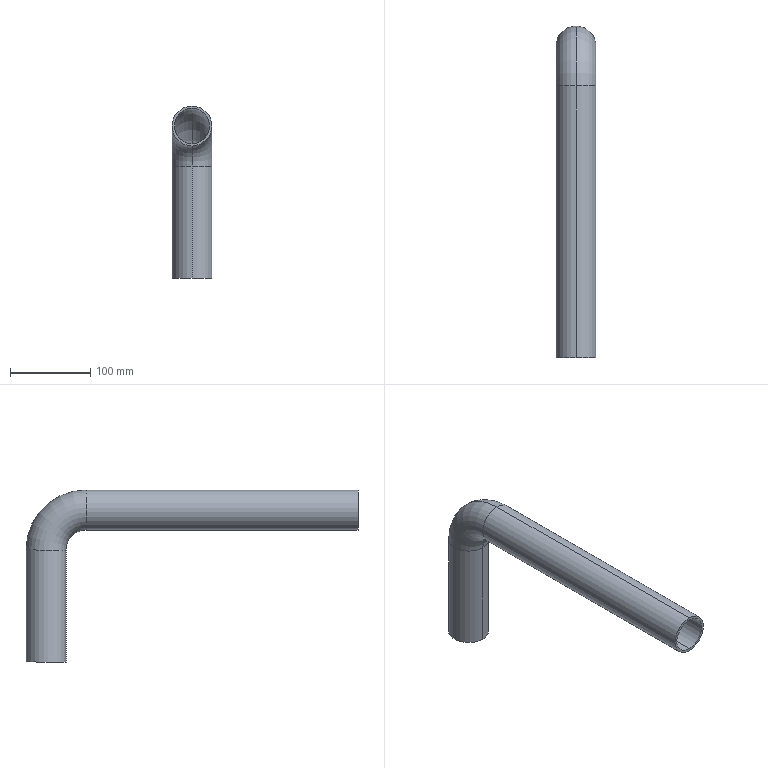Part | SolidWorks | features BaseBody 1 | 1 solid | 14 faces | box 50 x 415 x 215 mm | volume 247413 mm3 | cylinder 8 | torus 4 | plane 2 | commonest cylinder face diameters 44 x4 50 x4
STEP:
#1=CARTESIAN_POINT('',(0.,340.,-25.));
#2=VERTEX_POINT('',#1);
#3=CARTESIAN_POINT('',(0.,340.,25.));
#4=VERTEX_POINT('',#3);
#5=CARTESIAN_POINT('',(0.,340.,0.));
#6=DIRECTION('',(0.,1.,0.));
#7=DIRECTION('',(0.,0.,1.));
#8=AXIS2_PLACEMENT_3D('',#5,#6,#7);
#9=CIRCLE('',#8,25.);
#10=EDGE_CURVE('',#2,#4,#9,.T.);
#11=ORIENTED_EDGE('',*,*,#10,.T.);
#12=CARTESIAN_POINT('',(0.,415.,-50.));
#13=VERTEX_POINT('',#12);
#14=CARTESIAN_POINT('',(0.,340.,-50.));
#15=DIRECTION('',(-1.,0.,0.));
#16=DIRECTION('',(0.,0.,1.));
#17=AXIS2_PLACEMENT_3D('',#14,#15,#16);
#18=CIRCLE('',#17,75.);
#19=EDGE_CURVE('',#4,#13,#18,.T.);
#20=ORIENTED_EDGE('',*,*,#19,.T.);
#21=CARTESIAN_POINT('',(0.,365.,-50.));
#22=VERTEX_POINT('',#21);
#23=CARTESIAN_POINT('',(0.,390.,-50.));
#24=DIRECTION('',(0.,0.,-1.));
#25=DIRECTION('',(0.,1.,0.));
#26=AXIS2_PLACEMENT_3D('',#23,#24,#25);
#27=CIRCLE('',#26,25.);
#28=EDGE_CURVE('',#22,#13,#27,.T.);
#29=ORIENTED_EDGE('',*,*,#28,.F.);
#30=CARTESIAN_POINT('',(0.,340.,-50.));
#31=DIRECTION('',(-1.,0.,0.));
#32=DIRECTION('',(0.,0.,1.));
#33=AXIS2_PLACEMENT_3D('',#30,#31,#32);
#34=CIRCLE('',#33,25.);
#35=EDGE_CURVE('',#2,#22,#34,.T.);
#36=ORIENTED_EDGE('',*,*,#35,.F.);
#37=EDGE_LOOP('',(#11,#20,#29,#36));
#38=FACE_OUTER_BOUND('',#37,.T.);
#39=CARTESIAN_POINT('',(0.,340.,-50.));
#40=DIRECTION('',(-1.,0.,0.));
#41=DIRECTION('',(0.,0.,-1.));
#42=AXIS2_PLACEMENT_3D('',#39,#40,#41);
#43=TOROIDAL_SURFACE('',#42,50.,25.);
#44=ADVANCED_FACE('',(#38),#43,.T.);
#45=CARTESIAN_POINT('',(0.,340.,22.));
#46=VERTEX_POINT('',#45);
#47=CARTESIAN_POINT('',(0.,340.,-22.));
#48=VERTEX_POINT('',#47);
#49=CARTESIAN_POINT('',(0.,340.,0.));
#50=DIRECTION('',(0.,1.,0.));
#51=DIRECTION('',(0.,0.,1.));
#52=AXIS2_PLACEMENT_3D('',#49,#50,#51);
#53=CIRCLE('',#52,22.);
#54=EDGE_CURVE('',#46,#48,#53,.T.);
#55=ORIENTED_EDGE('',*,*,#54,.F.);
#56=CARTESIAN_POINT('',(0.,412.,-50.));
#57=VERTEX_POINT('',#56);
#58=CARTESIAN_POINT('',(0.,340.,-50.));
#59=DIRECTION('',(-1.,0.,0.));
#60=DIRECTION('',(0.,0.,1.));
#61=AXIS2_PLACEMENT_3D('',#58,#59,#60);
#62=CIRCLE('',#61,72.);
#63=EDGE_CURVE('',#46,#57,#62,.T.);
#64=ORIENTED_EDGE('',*,*,#63,.T.);
#65=CARTESIAN_POINT('',(0.,368.,-50.));
#66=VERTEX_POINT('',#65);
#67=CARTESIAN_POINT('',(0.,390.,-50.));
#68=DIRECTION('',(0.,0.,-1.));
#69=DIRECTION('',(0.,1.,0.));
#70=AXIS2_PLACEMENT_3D('',#67,#68,#69);
#71=CIRCLE('',#70,22.);
#72=EDGE_CURVE('',#57,#66,#71,.T.);
#73=ORIENTED_EDGE('',*,*,#72,.T.);
#74=CARTESIAN_POINT('',(0.,340.,-50.));
#75=DIRECTION('',(-1.,0.,0.));
#76=DIRECTION('',(0.,0.,1.));
#77=AXIS2_PLACEMENT_3D('',#74,#75,#76);
#78=CIRCLE('',#77,28.);
#79=EDGE_CURVE('',#48,#66,#78,.T.);
#80=ORIENTED_EDGE('',*,*,#79,.F.);
#81=EDGE_LOOP('',(#55,#64,#73,#80));
#82=FACE_OUTER_BOUND('',#81,.T.);
#83=CARTESIAN_POINT('',(0.,340.,-50.));
#84=DIRECTION('',(-1.,0.,0.));
#85=DIRECTION('',(0.,0.,-1.));
#86=AXIS2_PLACEMENT_3D('',#83,#84,#85);
#87=TOROIDAL_SURFACE('',#86,50.,22.);
#88=ADVANCED_FACE('',(#82),#87,.F.);
#89=ORIENTED_EDGE('',*,*,#28,.T.);
#90=CARTESIAN_POINT('',(0.,415.,-190.));
#91=VERTEX_POINT('',#90);
#92=CARTESIAN_POINT('',(0.,415.,-50.));
#93=DIRECTION('',(0.,0.,-1.));
#94=VECTOR('',#93,1000.);
#95=LINE('',#92,#94);
#96=EDGE_CURVE('',#13,#91,#95,.T.);
#97=ORIENTED_EDGE('',*,*,#96,.T.);
#98=CARTESIAN_POINT('',(0.,365.,-190.));
#99=VERTEX_POINT('',#98);
#100=CARTESIAN_POINT('',(0.,390.,-190.));
#101=DIRECTION('',(0.,0.,-1.));
#102=DIRECTION('',(0.,1.,0.));
#103=AXIS2_PLACEMENT_3D('',#100,#101,#102);
#104=CIRCLE('',#103,25.);
#105=EDGE_CURVE('',#99,#91,#104,.T.);
#106=ORIENTED_EDGE('',*,*,#105,.F.);
#107=CARTESIAN_POINT('',(0.,365.,-50.));
#108=DIRECTION('',(0.,0.,-1.));
#109=VECTOR('',#108,1000.);
#110=LINE('',#107,#109);
#111=EDGE_CURVE('',#22,#99,#110,.T.);
#112=ORIENTED_EDGE('',*,*,#111,.F.);
#113=EDGE_LOOP('',(#89,#97,#106,#112));
#114=FACE_OUTER_BOUND('',#113,.T.);
#115=CARTESIAN_POINT('',(0.,390.,-50.));
#116=DIRECTION('',(0.,0.,-1.));
#117=DIRECTION('',(0.,-1.,0.));
#118=AXIS2_PLACEMENT_3D('',#115,#116,#117);
#119=CYLINDRICAL_SURFACE('',#118,25.);
#120=ADVANCED_FACE('',(#114),#119,.T.);
#121=ORIENTED_EDGE('',*,*,#72,.F.);
#122=CARTESIAN_POINT('',(0.,412.,-190.));
#123=VERTEX_POINT('',#122);
#124=CARTESIAN_POINT('',(0.,412.,-50.));
#125=DIRECTION('',(0.,0.,-1.));
#126=VECTOR('',#125,1000.);
#127=LINE('',#124,#126);
#128=EDGE_CURVE('',#57,#123,#127,.T.);
#129=ORIENTED_EDGE('',*,*,#128,.T.);
#130=CARTESIAN_POINT('',(0.,368.,-190.));
#131=VERTEX_POINT('',#130);
#132=CARTESIAN_POINT('',(0.,390.,-190.));
#133=DIRECTION('',(0.,0.,-1.));
#134=DIRECTION('',(0.,1.,0.));
#135=AXIS2_PLACEMENT_3D('',#132,#133,#134);
#136=CIRCLE('',#135,22.);
#137=EDGE_CURVE('',#123,#131,#136,.T.);
#138=ORIENTED_EDGE('',*,*,#137,.T.);
#139=CARTESIAN_POINT('',(0.,368.,-50.));
#140=DIRECTION('',(0.,0.,-1.));
#141=VECTOR('',#140,1000.);
#142=LINE('',#139,#141);
#143=EDGE_CURVE('',#66,#131,#142,.T.);
#144=ORIENTED_EDGE('',*,*,#143,.F.);
#145=EDGE_LOOP('',(#121,#129,#138,#144));
#146=FACE_OUTER_BOUND('',#145,.T.);
#147=CARTESIAN_POINT('',(0.,390.,-50.));
#148=DIRECTION('',(0.,0.,-1.));
#149=DIRECTION('',(0.,-1.,0.));
#150=AXIS2_PLACEMENT_3D('',#147,#148,#149);
#151=CYLINDRICAL_SURFACE('',#150,22.);
#152=ADVANCED_FACE('',(#146),#151,.F.);
#153=ORIENTED_EDGE('',*,*,#54,.T.);
#154=CARTESIAN_POINT('',(0.,0.,-22.));
#155=VERTEX_POINT('',#154);
#156=CARTESIAN_POINT('',(0.,340.,-22.));
#157=DIRECTION('',(0.,-1.,0.));
#158=VECTOR('',#157,1000.);
#159=LINE('',#156,#158);
#160=EDGE_CURVE('',#48,#155,#159,.T.);
#161=ORIENTED_EDGE('',*,*,#160,.T.);
#162=CARTESIAN_POINT('',(0.,0.,22.));
#163=VERTEX_POINT('',#162);
#164=CARTESIAN_POINT('',(0.,0.,0.));
#165=DIRECTION('',(0.,1.,0.));
#166=DIRECTION('',(0.,0.,1.));
#167=AXIS2_PLACEMENT_3D('',#164,#165,#166);
#168=CIRCLE('',#167,22.);
#169=EDGE_CURVE('',#163,#155,#168,.T.);
#170=ORIENTED_EDGE('',*,*,#169,.F.);
#171=CARTESIAN_POINT('',(0.,340.,22.));
#172=DIRECTION('',(0.,-1.,0.));
#173=VECTOR('',#172,1000.);
#174=LINE('',#171,#173);
#175=EDGE_CURVE('',#46,#163,#174,.T.);
#176=ORIENTED_EDGE('',*,*,#175,.F.);
#177=EDGE_LOOP('',(#153,#161,#170,#176));
#178=FACE_OUTER_BOUND('',#177,.T.);
#179=CARTESIAN_POINT('',(0.,340.,0.));
#180=DIRECTION('',(0.,-1.,0.));
#181=DIRECTION('',(0.,0.,1.));
#182=AXIS2_PLACEMENT_3D('',#179,#180,#181);
#183=CYLINDRICAL_SURFACE('',#182,22.);
#184=ADVANCED_FACE('',(#178),#183,.F.);
#185=ORIENTED_EDGE('',*,*,#10,.F.);
#186=CARTESIAN_POINT('',(0.,0.,-25.));
#187=VERTEX_POINT('',#186);
#188=CARTESIAN_POINT('',(0.,340.,-25.));
#189=DIRECTION('',(0.,-1.,0.));
#190=VECTOR('',#189,1000.);
#191=LINE('',#188,#190);
#192=EDGE_CURVE('',#2,#187,#191,.T.);
#193=ORIENTED_EDGE('',*,*,#192,.T.);
#194=CARTESIAN_POINT('',(0.,0.,25.));
#195=VERTEX_POINT('',#194);
#196=CARTESIAN_POINT('',(0.,0.,0.));
#197=DIRECTION('',(0.,1.,0.));
#198=DIRECTION('',(0.,0.,1.));
#199=AXIS2_PLACEMENT_3D('',#196,#197,#198);
#200=CIRCLE('',#199,25.);
#201=EDGE_CURVE('',#187,#195,#200,.T.);
#202=ORIENTED_EDGE('',*,*,#201,.T.);
#203=CARTESIAN_POINT('',(0.,340.,25.));
#204=DIRECTION('',(0.,-1.,0.));
#205=VECTOR('',#204,1000.);
#206=LINE('',#203,#205);
#207=EDGE_CURVE('',#4,#195,#206,.T.);
#208=ORIENTED_EDGE('',*,*,#207,.F.);
#209=EDGE_LOOP('',(#185,#193,#202,#208));
#210=FACE_OUTER_BOUND('',#209,.T.);
#211=CARTESIAN_POINT('',(0.,340.,0.));
#212=DIRECTION('',(0.,-1.,0.));
#213=DIRECTION('',(0.,0.,1.));
#214=AXIS2_PLACEMENT_3D('',#211,#212,#213);
#215=CYLINDRICAL_SURFACE('',#214,25.);
#216=ADVANCED_FACE('',(#210),#215,.T.);
#217=CARTESIAN_POINT('',(0.,0.,0.));
#218=DIRECTION('',(0.,1.,0.));
#219=DIRECTION('',(0.,0.,1.));
#220=AXIS2_PLACEMENT_3D('',#217,#218,#219);
#221=CIRCLE('',#220,25.);
#222=EDGE_CURVE('',#195,#187,#221,.T.);
#223=ORIENTED_EDGE('',*,*,#222,.F.);
#224=ORIENTED_EDGE('',*,*,#201,.F.);
#225=EDGE_LOOP('',(#223,#224));
#226=FACE_OUTER_BOUND('',#225,.T.);
#227=ORIENTED_EDGE('',*,*,#169,.T.);
#228=CARTESIAN_POINT('',(0.,0.,0.));
#229=DIRECTION('',(0.,1.,0.));
#230=DIRECTION('',(0.,0.,1.));
#231=AXIS2_PLACEMENT_3D('',#228,#229,#230);
#232=CIRCLE('',#231,22.);
#233=EDGE_CURVE('',#155,#163,#232,.T.);
#234=ORIENTED_EDGE('',*,*,#233,.T.);
#235=EDGE_LOOP('',(#227,#234));
#236=FACE_BOUND('',#235,.T.);
#237=CARTESIAN_POINT('',(0.,0.,0.));
#238=DIRECTION('',(0.,1.,0.));
#239=DIRECTION('',(1.,0.,0.));
#240=AXIS2_PLACEMENT_3D('',#237,#238,#239);
#241=PLANE('',#240);
#242=ADVANCED_FACE('',(#226,#236),#241,.F.);
#243=ORIENTED_EDGE('',*,*,#105,.T.);
#244=CARTESIAN_POINT('',(0.,390.,-190.));
#245=DIRECTION('',(0.,0.,-1.));
#246=DIRECTION('',(0.,1.,0.));
#247=AXIS2_PLACEMENT_3D('',#244,#245,#246);
#248=CIRCLE('',#247,25.);
#249=EDGE_CURVE('',#91,#99,#248,.T.);
#250=ORIENTED_EDGE('',*,*,#249,.T.);
#251=EDGE_LOOP('',(#243,#250));
#252=FACE_OUTER_BOUND('',#251,.T.);
#253=CARTESIAN_POINT('',(0.,390.,-190.));
#254=DIRECTION('',(0.,0.,-1.));
#255=DIRECTION('',(0.,1.,0.));
#256=AXIS2_PLACEMENT_3D('',#253,#254,#255);
#257=CIRCLE('',#256,22.);
#258=EDGE_CURVE('',#131,#123,#257,.T.);
#259=ORIENTED_EDGE('',*,*,#258,.F.);
#260=ORIENTED_EDGE('',*,*,#137,.F.);
#261=EDGE_LOOP('',(#259,#260));
#262=FACE_BOUND('',#261,.T.);
#263=CARTESIAN_POINT('',(0.,390.,-190.));
#264=DIRECTION('',(0.,0.,-1.));
#265=DIRECTION('',(-1.,0.,0.));
#266=AXIS2_PLACEMENT_3D('',#263,#264,#265);
#267=PLANE('',#266);
#268=ADVANCED_FACE('',(#252,#262),#267,.T.);
#269=ORIENTED_EDGE('',*,*,#192,.F.);
#270=CARTESIAN_POINT('',(0.,340.,0.));
#271=DIRECTION('',(0.,1.,0.));
#272=DIRECTION('',(0.,0.,1.));
#273=AXIS2_PLACEMENT_3D('',#270,#271,#272);
#274=CIRCLE('',#273,25.);
#275=EDGE_CURVE('',#4,#2,#274,.T.);
#276=ORIENTED_EDGE('',*,*,#275,.F.);
#277=ORIENTED_EDGE('',*,*,#207,.T.);
#278=ORIENTED_EDGE('',*,*,#222,.T.);
#279=EDGE_LOOP('',(#269,#276,#277,#278));
#280=FACE_OUTER_BOUND('',#279,.T.);
#281=CARTESIAN_POINT('',(0.,340.,0.));
#282=DIRECTION('',(0.,-1.,0.));
#283=DIRECTION('',(0.,0.,1.));
#284=AXIS2_PLACEMENT_3D('',#281,#282,#283);
#285=CYLINDRICAL_SURFACE('',#284,25.);
#286=ADVANCED_FACE('',(#280),#285,.T.);
#287=ORIENTED_EDGE('',*,*,#160,.F.);
#288=CARTESIAN_POINT('',(0.,340.,0.));
#289=DIRECTION('',(0.,1.,0.));
#290=DIRECTION('',(0.,0.,1.));
#291=AXIS2_PLACEMENT_3D('',#288,#289,#290);
#292=CIRCLE('',#291,22.);
#293=EDGE_CURVE('',#48,#46,#292,.T.);
#294=ORIENTED_EDGE('',*,*,#293,.T.);
#295=ORIENTED_EDGE('',*,*,#175,.T.);
#296=ORIENTED_EDGE('',*,*,#233,.F.);
#297=EDGE_LOOP('',(#287,#294,#295,#296));
#298=FACE_OUTER_BOUND('',#297,.T.);
#299=CARTESIAN_POINT('',(0.,340.,0.));
#300=DIRECTION('',(0.,-1.,0.));
#301=DIRECTION('',(0.,0.,1.));
#302=AXIS2_PLACEMENT_3D('',#299,#300,#301);
#303=CYLINDRICAL_SURFACE('',#302,22.);
#304=ADVANCED_FACE('',(#298),#303,.F.);
#305=ORIENTED_EDGE('',*,*,#63,.F.);
#306=ORIENTED_EDGE('',*,*,#293,.F.);
#307=ORIENTED_EDGE('',*,*,#79,.T.);
#308=CARTESIAN_POINT('',(0.,390.,-50.));
#309=DIRECTION('',(0.,0.,-1.));
#310=DIRECTION('',(0.,1.,0.));
#311=AXIS2_PLACEMENT_3D('',#308,#309,#310);
#312=CIRCLE('',#311,22.);
#313=EDGE_CURVE('',#66,#57,#312,.T.);
#314=ORIENTED_EDGE('',*,*,#313,.T.);
#315=EDGE_LOOP('',(#305,#306,#307,#314));
#316=FACE_OUTER_BOUND('',#315,.T.);
#317=CARTESIAN_POINT('',(0.,340.,-50.));
#318=DIRECTION('',(-1.,0.,0.));
#319=DIRECTION('',(0.,0.,-1.));
#320=AXIS2_PLACEMENT_3D('',#317,#318,#319);
#321=TOROIDAL_SURFACE('',#320,50.,22.);
#322=ADVANCED_FACE('',(#316),#321,.F.);
#323=ORIENTED_EDGE('',*,*,#19,.F.);
#324=ORIENTED_EDGE('',*,*,#275,.T.);
#325=ORIENTED_EDGE('',*,*,#35,.T.);
#326=CARTESIAN_POINT('',(0.,390.,-50.));
#327=DIRECTION('',(0.,0.,-1.));
#328=DIRECTION('',(0.,1.,0.));
#329=AXIS2_PLACEMENT_3D('',#326,#327,#328);
#330=CIRCLE('',#329,25.);
#331=EDGE_CURVE('',#13,#22,#330,.T.);
#332=ORIENTED_EDGE('',*,*,#331,.F.);
#333=EDGE_LOOP('',(#323,#324,#325,#332));
#334=FACE_OUTER_BOUND('',#333,.T.);
#335=CARTESIAN_POINT('',(0.,340.,-50.));
#336=DIRECTION('',(-1.,0.,0.));
#337=DIRECTION('',(0.,0.,-1.));
#338=AXIS2_PLACEMENT_3D('',#335,#336,#337);
#339=TOROIDAL_SURFACE('',#338,50.,25.);
#340=ADVANCED_FACE('',(#334),#339,.T.);
#341=ORIENTED_EDGE('',*,*,#128,.F.);
#342=ORIENTED_EDGE('',*,*,#313,.F.);
#343=ORIENTED_EDGE('',*,*,#143,.T.);
#344=ORIENTED_EDGE('',*,*,#258,.T.);
#345=EDGE_LOOP('',(#341,#342,#343,#344));
#346=FACE_OUTER_BOUND('',#345,.T.);
#347=CARTESIAN_POINT('',(0.,390.,-50.));
#348=DIRECTION('',(0.,0.,-1.));
#349=DIRECTION('',(0.,-1.,0.));
#350=AXIS2_PLACEMENT_3D('',#347,#348,#349);
#351=CYLINDRICAL_SURFACE('',#350,22.);
#352=ADVANCED_FACE('',(#346),#351,.F.);
#353=ORIENTED_EDGE('',*,*,#96,.F.);
#354=ORIENTED_EDGE('',*,*,#331,.T.);
#355=ORIENTED_EDGE('',*,*,#111,.T.);
#356=ORIENTED_EDGE('',*,*,#249,.F.);
#357=EDGE_LOOP('',(#353,#354,#355,#356));
#358=FACE_OUTER_BOUND('',#357,.T.);
#359=CARTESIAN_POINT('',(0.,390.,-50.));
#360=DIRECTION('',(0.,0.,-1.));
#361=DIRECTION('',(0.,-1.,0.));
#362=AXIS2_PLACEMENT_3D('',#359,#360,#361);
#363=CYLINDRICAL_SURFACE('',#362,25.);
#364=ADVANCED_FACE('',(#358),#363,.T.);
#365=CLOSED_SHELL('',(#44,#88,#120,#152,#184,#216,#242,#268,#286,#304,#322,#340,#352,#364));
#366=MANIFOLD_SOLID_BREP('',#365);
#367=CARTESIAN_POINT('',(0.,0.,0.));
#368=DIRECTION('',(0.,0.,1.));
#369=DIRECTION('',(1.,0.,0.));
#370=AXIS2_PLACEMENT_3D('',#367,#368,#369);
#371=(LENGTH_UNIT()NAMED_UNIT(*)SI_UNIT(.MILLI.,.METRE.));
#372=UNCERTAINTY_MEASURE_WITH_UNIT(LENGTH_MEASURE(0.00001),#371,'','');
#373=(NAMED_UNIT(*)PLANE_ANGLE_UNIT()SI_UNIT($,.RADIAN.));
#374=(NAMED_UNIT(*)SI_UNIT($,.STERADIAN.)SOLID_ANGLE_UNIT());
#375=(GEOMETRIC_REPRESENTATION_CONTEXT(3)GLOBAL_UNCERTAINTY_ASSIGNED_CONTEXT((#372))GLOBAL_UNIT_ASSIGNED_CONTEXT((#371,#373,#374))REPRESENTATION_CONTEXT('',''));
#376=ADVANCED_BREP_SHAPE_REPRESENTATION('',(#366,#370),#375);